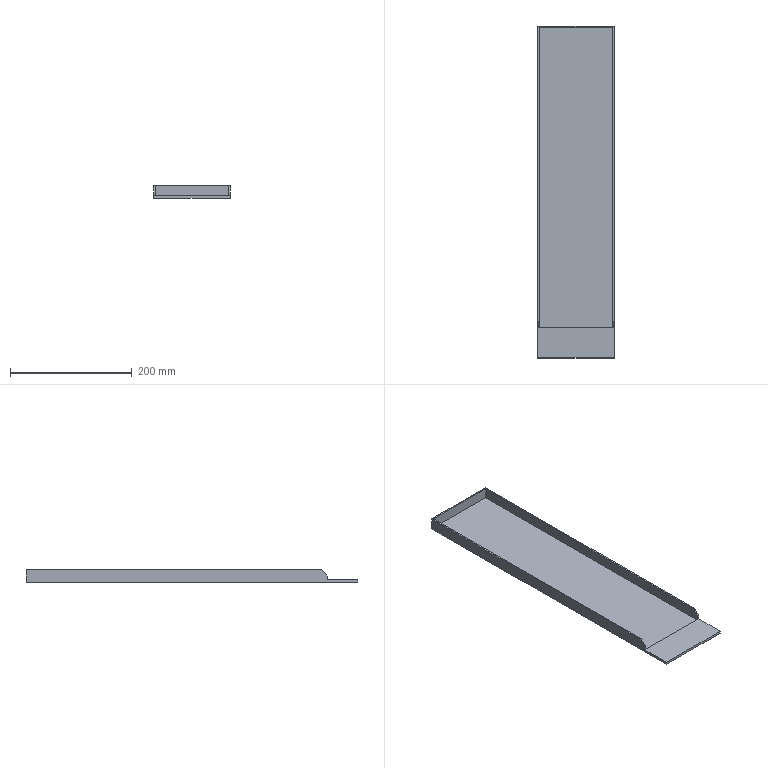Part | NX | features solid 2 | 1 solid | 16 faces | box 125 x 545 x 20 mm | volume 188546 mm3 | plane 16
STEP:
#1=CARTESIAN_POINT('',(-227.,-415.,-318.));
#2=VERTEX_POINT('',#1);
#3=CARTESIAN_POINT('',(-227.,78.,-318.));
#4=VERTEX_POINT('',#3);
#5=CARTESIAN_POINT('',(-227.,-415.,-318.));
#6=DIRECTION('',(0.,1.,0.));
#7=VECTOR('',#6,1000.);
#8=LINE('',#5,#7);
#9=EDGE_CURVE('',#2,#4,#8,.T.);
#10=ORIENTED_EDGE('',*,*,#9,.T.);
#11=CARTESIAN_POINT('',(-348.,78.,-318.));
#12=VERTEX_POINT('',#11);
#13=CARTESIAN_POINT('',(-350.,78.,-318.));
#14=DIRECTION('',(-1.,0.,0.));
#15=VECTOR('',#14,1000.);
#16=LINE('',#13,#15);
#17=EDGE_CURVE('',#12,#4,#16,.F.);
#18=ORIENTED_EDGE('',*,*,#17,.F.);
#19=CARTESIAN_POINT('',(-348.,-415.,-318.));
#20=VERTEX_POINT('',#19);
#21=CARTESIAN_POINT('',(-348.,78.,-318.));
#22=DIRECTION('',(0.,1.,0.));
#23=VECTOR('',#22,1000.);
#24=LINE('',#21,#23);
#25=EDGE_CURVE('',#12,#20,#24,.F.);
#26=ORIENTED_EDGE('',*,*,#25,.T.);
#27=CARTESIAN_POINT('',(-350.,-415.,-318.));
#28=DIRECTION('',(1.,0.,0.));
#29=VECTOR('',#28,1000.);
#30=LINE('',#27,#29);
#31=EDGE_CURVE('',#20,#2,#30,.T.);
#32=ORIENTED_EDGE('',*,*,#31,.T.);
#33=EDGE_LOOP('',(#10,#18,#26,#32));
#34=FACE_BOUND('',#33,.T.);
#35=CARTESIAN_POINT('',(-350.,-70.,-318.));
#36=DIRECTION('',(0.,0.,-1.));
#37=DIRECTION('',(-1.,0.,0.));
#38=AXIS2_PLACEMENT_3D('',#35,#36,#37);
#39=PLANE('',#38);
#40=ADVANCED_FACE('',(#34),#39,.F.);
#41=CARTESIAN_POINT('',(-225.,80.,-320.));
#42=VERTEX_POINT('',#41);
#43=CARTESIAN_POINT('',(-350.,80.,-320.));
#44=VERTEX_POINT('',#43);
#45=CARTESIAN_POINT('',(-350.,80.,-320.));
#46=DIRECTION('',(-1.,0.,0.));
#47=VECTOR('',#46,1000.);
#48=LINE('',#45,#47);
#49=EDGE_CURVE('',#42,#44,#48,.T.);
#50=ORIENTED_EDGE('',*,*,#49,.T.);
#51=CARTESIAN_POINT('',(-350.,80.,-300.));
#52=VERTEX_POINT('',#51);
#53=CARTESIAN_POINT('',(-350.,80.,-318.));
#54=DIRECTION('',(0.,0.,-1.));
#55=VECTOR('',#54,1000.);
#56=LINE('',#53,#55);
#57=EDGE_CURVE('',#52,#44,#56,.T.);
#58=ORIENTED_EDGE('',*,*,#57,.F.);
#59=CARTESIAN_POINT('',(-225.,80.,-300.));
#60=VERTEX_POINT('',#59);
#61=CARTESIAN_POINT('',(-380.,80.,-300.));
#62=DIRECTION('',(1.,0.,0.));
#63=VECTOR('',#62,1000.);
#64=LINE('',#61,#63);
#65=EDGE_CURVE('',#60,#52,#64,.F.);
#66=ORIENTED_EDGE('',*,*,#65,.F.);
#67=CARTESIAN_POINT('',(-225.,80.,-318.));
#68=DIRECTION('',(0.,0.,-1.));
#69=VECTOR('',#68,1000.);
#70=LINE('',#67,#69);
#71=EDGE_CURVE('',#60,#42,#70,.T.);
#72=ORIENTED_EDGE('',*,*,#71,.T.);
#73=EDGE_LOOP('',(#50,#58,#66,#72));
#74=FACE_BOUND('',#73,.T.);
#75=CARTESIAN_POINT('',(-350.,80.,-318.));
#76=DIRECTION('',(0.,-1.,0.));
#77=DIRECTION('',(0.,0.,-1.));
#78=AXIS2_PLACEMENT_3D('',#75,#76,#77);
#79=PLANE('',#78);
#80=ADVANCED_FACE('',(#74),#79,.F.);
#81=CARTESIAN_POINT('',(-225.,-405.,-300.));
#82=VERTEX_POINT('',#81);
#83=CARTESIAN_POINT('',(-225.,-15.,-300.));
#84=DIRECTION('',(0.,-1.,0.));
#85=VECTOR('',#84,1000.);
#86=LINE('',#83,#85);
#87=EDGE_CURVE('',#82,#60,#86,.F.);
#88=ORIENTED_EDGE('',*,*,#87,.F.);
#89=CARTESIAN_POINT('',(-225.,-415.,-310.));
#90=VERTEX_POINT('',#89);
#91=CARTESIAN_POINT('',(-225.,-415.,-310.));
#92=DIRECTION('',(0.,0.7071,0.7071));
#93=VECTOR('',#92,1000.);
#94=LINE('',#91,#93);
#95=EDGE_CURVE('',#82,#90,#94,.F.);
#96=ORIENTED_EDGE('',*,*,#95,.T.);
#97=CARTESIAN_POINT('',(-225.,-415.,-316.));
#98=VERTEX_POINT('',#97);
#99=CARTESIAN_POINT('',(-225.,-415.,-298.));
#100=DIRECTION('',(0.,0.,-1.));
#101=VECTOR('',#100,1000.);
#102=LINE('',#99,#101);
#103=EDGE_CURVE('',#90,#98,#102,.T.);
#104=ORIENTED_EDGE('',*,*,#103,.T.);
#105=CARTESIAN_POINT('',(-225.,-465.,-316.));
#106=VERTEX_POINT('',#105);
#107=CARTESIAN_POINT('',(-225.,-415.,-316.));
#108=DIRECTION('',(0.,1.,0.));
#109=VECTOR('',#108,1000.);
#110=LINE('',#107,#109);
#111=EDGE_CURVE('',#98,#106,#110,.F.);
#112=ORIENTED_EDGE('',*,*,#111,.T.);
#113=CARTESIAN_POINT('',(-225.,-465.,-320.));
#114=VERTEX_POINT('',#113);
#115=CARTESIAN_POINT('',(-225.,-465.,-318.));
#116=DIRECTION('',(0.,0.,1.));
#117=VECTOR('',#116,1000.);
#118=LINE('',#115,#117);
#119=EDGE_CURVE('',#106,#114,#118,.F.);
#120=ORIENTED_EDGE('',*,*,#119,.T.);
#121=CARTESIAN_POINT('',(-225.,-70.,-320.));
#122=DIRECTION('',(0.,-1.,0.));
#123=VECTOR('',#122,1000.);
#124=LINE('',#121,#123);
#125=EDGE_CURVE('',#114,#42,#124,.F.);
#126=ORIENTED_EDGE('',*,*,#125,.T.);
#127=ORIENTED_EDGE('',*,*,#71,.F.);
#128=EDGE_LOOP('',(#88,#96,#104,#112,#120,#126,#127));
#129=FACE_BOUND('',#128,.T.);
#130=CARTESIAN_POINT('',(-225.,-70.,-318.));
#131=DIRECTION('',(-1.,0.,0.));
#132=DIRECTION('',(0.,0.,1.));
#133=AXIS2_PLACEMENT_3D('',#130,#131,#132);
#134=PLANE('',#133);
#135=ADVANCED_FACE('',(#129),#134,.F.);
#136=CARTESIAN_POINT('',(-350.,-465.,-320.));
#137=VERTEX_POINT('',#136);
#138=CARTESIAN_POINT('',(-910.,-465.,-320.));
#139=DIRECTION('',(1.,0.,0.));
#140=VECTOR('',#139,1000.);
#141=LINE('',#138,#140);
#142=EDGE_CURVE('',#137,#114,#141,.T.);
#143=ORIENTED_EDGE('',*,*,#142,.T.);
#144=ORIENTED_EDGE('',*,*,#119,.F.);
#145=CARTESIAN_POINT('',(-350.,-465.,-316.));
#146=VERTEX_POINT('',#145);
#147=CARTESIAN_POINT('',(-350.,-465.,-316.));
#148=DIRECTION('',(-1.,0.,0.));
#149=VECTOR('',#148,1000.);
#150=LINE('',#147,#149);
#151=EDGE_CURVE('',#146,#106,#150,.F.);
#152=ORIENTED_EDGE('',*,*,#151,.F.);
#153=CARTESIAN_POINT('',(-350.,-465.,-85.));
#154=DIRECTION('',(0.,0.,1.));
#155=VECTOR('',#154,1000.);
#156=LINE('',#153,#155);
#157=EDGE_CURVE('',#146,#137,#156,.F.);
#158=ORIENTED_EDGE('',*,*,#157,.T.);
#159=EDGE_LOOP('',(#143,#144,#152,#158));
#160=FACE_BOUND('',#159,.T.);
#161=CARTESIAN_POINT('',(-910.,-465.,-85.));
#162=DIRECTION('',(0.,-1.,0.));
#163=DIRECTION('',(0.,0.,-1.));
#164=AXIS2_PLACEMENT_3D('',#161,#162,#163);
#165=PLANE('',#164);
#166=ADVANCED_FACE('',(#160),#165,.T.);
#167=CARTESIAN_POINT('',(-350.,-415.,-310.));
#168=VERTEX_POINT('',#167);
#169=CARTESIAN_POINT('',(-350.,-415.,-316.));
#170=VERTEX_POINT('',#169);
#171=CARTESIAN_POINT('',(-350.,-415.,-298.));
#172=DIRECTION('',(0.,0.,-1.));
#173=VECTOR('',#172,1000.);
#174=LINE('',#171,#173);
#175=EDGE_CURVE('',#168,#170,#174,.T.);
#176=ORIENTED_EDGE('',*,*,#175,.F.);
#177=CARTESIAN_POINT('',(-350.,-405.,-300.));
#178=VERTEX_POINT('',#177);
#179=CARTESIAN_POINT('',(-350.,-400.,-295.));
#180=DIRECTION('',(0.,0.7071,0.7071));
#181=VECTOR('',#180,1000.);
#182=LINE('',#179,#181);
#183=EDGE_CURVE('',#168,#178,#182,.T.);
#184=ORIENTED_EDGE('',*,*,#183,.T.);
#185=CARTESIAN_POINT('',(-350.,-70.,-300.));
#186=DIRECTION('',(0.,-1.,0.));
#187=VECTOR('',#186,1000.);
#188=LINE('',#185,#187);
#189=EDGE_CURVE('',#178,#52,#188,.F.);
#190=ORIENTED_EDGE('',*,*,#189,.T.);
#191=ORIENTED_EDGE('',*,*,#57,.T.);
#192=CARTESIAN_POINT('',(-350.,-70.,-320.));
#193=DIRECTION('',(0.,1.,0.));
#194=VECTOR('',#193,1000.);
#195=LINE('',#192,#194);
#196=EDGE_CURVE('',#44,#137,#195,.F.);
#197=ORIENTED_EDGE('',*,*,#196,.T.);
#198=ORIENTED_EDGE('',*,*,#157,.F.);
#199=CARTESIAN_POINT('',(-350.,-415.,-316.));
#200=DIRECTION('',(0.,1.,0.));
#201=VECTOR('',#200,1000.);
#202=LINE('',#199,#201);
#203=EDGE_CURVE('',#170,#146,#202,.F.);
#204=ORIENTED_EDGE('',*,*,#203,.F.);
#205=EDGE_LOOP('',(#176,#184,#190,#191,#197,#198,#204));
#206=FACE_BOUND('',#205,.T.);
#207=CARTESIAN_POINT('',(-350.,-70.,-318.));
#208=DIRECTION('',(1.,0.,0.));
#209=DIRECTION('',(0.,0.,-1.));
#210=AXIS2_PLACEMENT_3D('',#207,#208,#209);
#211=PLANE('',#210);
#212=ADVANCED_FACE('',(#206),#211,.F.);
#213=ORIENTED_EDGE('',*,*,#142,.F.);
#214=ORIENTED_EDGE('',*,*,#196,.F.);
#215=ORIENTED_EDGE('',*,*,#49,.F.);
#216=ORIENTED_EDGE('',*,*,#125,.F.);
#217=EDGE_LOOP('',(#213,#214,#215,#216));
#218=FACE_BOUND('',#217,.T.);
#219=CARTESIAN_POINT('',(-350.,-70.,-320.));
#220=DIRECTION('',(0.,0.,-1.));
#221=DIRECTION('',(-1.,0.,0.));
#222=AXIS2_PLACEMENT_3D('',#219,#220,#221);
#223=PLANE('',#222);
#224=ADVANCED_FACE('',(#218),#223,.T.);
#225=CARTESIAN_POINT('',(-227.,-415.,-316.));
#226=VERTEX_POINT('',#225);
#227=CARTESIAN_POINT('',(-227.,-415.,-298.));
#228=DIRECTION('',(0.,0.,1.));
#229=VECTOR('',#228,1000.);
#230=LINE('',#227,#229);
#231=EDGE_CURVE('',#226,#2,#230,.F.);
#232=ORIENTED_EDGE('',*,*,#231,.T.);
#233=ORIENTED_EDGE('',*,*,#31,.F.);
#234=CARTESIAN_POINT('',(-348.,-415.,-316.));
#235=VERTEX_POINT('',#234);
#236=CARTESIAN_POINT('',(-348.,-415.,-298.));
#237=DIRECTION('',(0.,0.,-1.));
#238=VECTOR('',#237,1000.);
#239=LINE('',#236,#238);
#240=EDGE_CURVE('',#235,#20,#239,.T.);
#241=ORIENTED_EDGE('',*,*,#240,.F.);
#242=CARTESIAN_POINT('',(-350.,-415.,-316.));
#243=DIRECTION('',(-1.,0.,0.));
#244=VECTOR('',#243,1000.);
#245=LINE('',#242,#244);
#246=EDGE_CURVE('',#235,#226,#245,.F.);
#247=ORIENTED_EDGE('',*,*,#246,.T.);
#248=EDGE_LOOP('',(#232,#233,#241,#247));
#249=FACE_BOUND('',#248,.T.);
#250=CARTESIAN_POINT('',(-350.,-415.,-318.));
#251=DIRECTION('',(0.,1.,0.));
#252=DIRECTION('',(1.,0.,0.));
#253=AXIS2_PLACEMENT_3D('',#250,#251,#252);
#254=PLANE('',#253);
#255=ADVANCED_FACE('',(#249),#254,.T.);
#256=ORIENTED_EDGE('',*,*,#151,.T.);
#257=ORIENTED_EDGE('',*,*,#111,.F.);
#258=CARTESIAN_POINT('',(-350.,-415.,-316.));
#259=DIRECTION('',(-1.,0.,0.));
#260=VECTOR('',#259,1000.);
#261=LINE('',#258,#260);
#262=EDGE_CURVE('',#226,#98,#261,.F.);
#263=ORIENTED_EDGE('',*,*,#262,.F.);
#264=ORIENTED_EDGE('',*,*,#246,.F.);
#265=CARTESIAN_POINT('',(-350.,-415.,-316.));
#266=DIRECTION('',(-1.,0.,0.));
#267=VECTOR('',#266,1000.);
#268=LINE('',#265,#267);
#269=EDGE_CURVE('',#170,#235,#268,.F.);
#270=ORIENTED_EDGE('',*,*,#269,.F.);
#271=ORIENTED_EDGE('',*,*,#203,.T.);
#272=EDGE_LOOP('',(#256,#257,#263,#264,#270,#271));
#273=FACE_BOUND('',#272,.T.);
#274=CARTESIAN_POINT('',(-350.,-415.,-316.));
#275=DIRECTION('',(0.,0.,-1.));
#276=DIRECTION('',(-1.,0.,0.));
#277=AXIS2_PLACEMENT_3D('',#274,#275,#276);
#278=PLANE('',#277);
#279=ADVANCED_FACE('',(#273),#278,.F.);
#280=CARTESIAN_POINT('',(-227.,78.,-300.));
#281=VERTEX_POINT('',#280);
#282=CARTESIAN_POINT('',(-227.,78.,-298.));
#283=DIRECTION('',(0.,0.,1.));
#284=VECTOR('',#283,1000.);
#285=LINE('',#282,#284);
#286=EDGE_CURVE('',#281,#4,#285,.F.);
#287=ORIENTED_EDGE('',*,*,#286,.F.);
#288=CARTESIAN_POINT('',(-348.,78.,-300.));
#289=VERTEX_POINT('',#288);
#290=CARTESIAN_POINT('',(-380.,78.,-300.));
#291=DIRECTION('',(1.,0.,0.));
#292=VECTOR('',#291,1000.);
#293=LINE('',#290,#292);
#294=EDGE_CURVE('',#281,#289,#293,.F.);
#295=ORIENTED_EDGE('',*,*,#294,.T.);
#296=CARTESIAN_POINT('',(-348.,78.,-298.));
#297=DIRECTION('',(0.,0.,-1.));
#298=VECTOR('',#297,1000.);
#299=LINE('',#296,#298);
#300=EDGE_CURVE('',#289,#12,#299,.T.);
#301=ORIENTED_EDGE('',*,*,#300,.T.);
#302=ORIENTED_EDGE('',*,*,#17,.T.);
#303=EDGE_LOOP('',(#287,#295,#301,#302));
#304=FACE_BOUND('',#303,.T.);
#305=CARTESIAN_POINT('',(-225.,78.,-318.));
#306=DIRECTION('',(0.,-1.,0.));
#307=DIRECTION('',(-1.,0.,0.));
#308=AXIS2_PLACEMENT_3D('',#305,#306,#307);
#309=PLANE('',#308);
#310=ADVANCED_FACE('',(#304),#309,.T.);
#311=CARTESIAN_POINT('',(-227.,-405.,-300.));
#312=VERTEX_POINT('',#311);
#313=CARTESIAN_POINT('',(-227.,-15.,-300.));
#314=DIRECTION('',(0.,-1.,0.));
#315=VECTOR('',#314,1000.);
#316=LINE('',#313,#315);
#317=EDGE_CURVE('',#312,#281,#316,.F.);
#318=ORIENTED_EDGE('',*,*,#317,.F.);
#319=CARTESIAN_POINT('',(-225.,-405.,-300.));
#320=DIRECTION('',(1.,0.,0.));
#321=VECTOR('',#320,1000.);
#322=LINE('',#319,#321);
#323=EDGE_CURVE('',#312,#82,#322,.T.);
#324=ORIENTED_EDGE('',*,*,#323,.T.);
#325=ORIENTED_EDGE('',*,*,#87,.T.);
#326=ORIENTED_EDGE('',*,*,#65,.T.);
#327=ORIENTED_EDGE('',*,*,#189,.F.);
#328=CARTESIAN_POINT('',(-348.,-405.,-300.));
#329=VERTEX_POINT('',#328);
#330=CARTESIAN_POINT('',(-225.,-405.,-300.));
#331=DIRECTION('',(-1.,0.,0.));
#332=VECTOR('',#331,1000.);
#333=LINE('',#330,#332);
#334=EDGE_CURVE('',#178,#329,#333,.F.);
#335=ORIENTED_EDGE('',*,*,#334,.T.);
#336=CARTESIAN_POINT('',(-348.,-15.,-300.));
#337=DIRECTION('',(0.,1.,0.));
#338=VECTOR('',#337,1000.);
#339=LINE('',#336,#338);
#340=EDGE_CURVE('',#289,#329,#339,.F.);
#341=ORIENTED_EDGE('',*,*,#340,.F.);
#342=ORIENTED_EDGE('',*,*,#294,.F.);
#343=EDGE_LOOP('',(#318,#324,#325,#326,#327,#335,#341,#342));
#344=FACE_BOUND('',#343,.T.);
#345=CARTESIAN_POINT('',(-380.,-15.,-300.));
#346=DIRECTION('',(0.,0.,1.));
#347=DIRECTION('',(1.,0.,0.));
#348=AXIS2_PLACEMENT_3D('',#345,#346,#347);
#349=PLANE('',#348);
#350=ADVANCED_FACE('',(#344),#349,.T.);
#351=CARTESIAN_POINT('',(-348.,-415.,-310.));
#352=VERTEX_POINT('',#351);
#353=CARTESIAN_POINT('',(-348.,-415.,-298.));
#354=DIRECTION('',(0.,0.,-1.));
#355=VECTOR('',#354,1000.);
#356=LINE('',#353,#355);
#357=EDGE_CURVE('',#352,#235,#356,.T.);
#358=ORIENTED_EDGE('',*,*,#357,.F.);
#359=CARTESIAN_POINT('',(-350.,-415.,-310.));
#360=DIRECTION('',(1.,0.,0.));
#361=VECTOR('',#360,1000.);
#362=LINE('',#359,#361);
#363=EDGE_CURVE('',#352,#168,#362,.F.);
#364=ORIENTED_EDGE('',*,*,#363,.T.);
#365=ORIENTED_EDGE('',*,*,#175,.T.);
#366=ORIENTED_EDGE('',*,*,#269,.T.);
#367=EDGE_LOOP('',(#358,#364,#365,#366));
#368=FACE_BOUND('',#367,.T.);
#369=CARTESIAN_POINT('',(-350.,-415.,-298.));
#370=DIRECTION('',(0.,-1.,0.));
#371=DIRECTION('',(0.,0.,-1.));
#372=AXIS2_PLACEMENT_3D('',#369,#370,#371);
#373=PLANE('',#372);
#374=ADVANCED_FACE('',(#368),#373,.T.);
#375=ORIENTED_EDGE('',*,*,#340,.T.);
#376=CARTESIAN_POINT('',(-348.,-162.5,-57.5));
#377=DIRECTION('',(0.,-0.7071,-0.7071));
#378=VECTOR('',#377,1000.);
#379=LINE('',#376,#378);
#380=EDGE_CURVE('',#329,#352,#379,.T.);
#381=ORIENTED_EDGE('',*,*,#380,.T.);
#382=ORIENTED_EDGE('',*,*,#357,.T.);
#383=ORIENTED_EDGE('',*,*,#240,.T.);
#384=ORIENTED_EDGE('',*,*,#25,.F.);
#385=ORIENTED_EDGE('',*,*,#300,.F.);
#386=EDGE_LOOP('',(#375,#381,#382,#383,#384,#385));
#387=FACE_BOUND('',#386,.T.);
#388=CARTESIAN_POINT('',(-348.,78.,-298.));
#389=DIRECTION('',(1.,0.,0.));
#390=DIRECTION('',(0.,0.,-1.));
#391=AXIS2_PLACEMENT_3D('',#388,#389,#390);
#392=PLANE('',#391);
#393=ADVANCED_FACE('',(#387),#392,.T.);
#394=ORIENTED_EDGE('',*,*,#103,.F.);
#395=CARTESIAN_POINT('',(-227.,-415.,-310.));
#396=VERTEX_POINT('',#395);
#397=CARTESIAN_POINT('',(-225.,-415.,-310.));
#398=DIRECTION('',(-1.,0.,0.));
#399=VECTOR('',#398,1000.);
#400=LINE('',#397,#399);
#401=EDGE_CURVE('',#90,#396,#400,.T.);
#402=ORIENTED_EDGE('',*,*,#401,.T.);
#403=CARTESIAN_POINT('',(-227.,-415.,-298.));
#404=DIRECTION('',(0.,0.,1.));
#405=VECTOR('',#404,1000.);
#406=LINE('',#403,#405);
#407=EDGE_CURVE('',#396,#226,#406,.F.);
#408=ORIENTED_EDGE('',*,*,#407,.T.);
#409=ORIENTED_EDGE('',*,*,#262,.T.);
#410=EDGE_LOOP('',(#394,#402,#408,#409));
#411=FACE_BOUND('',#410,.T.);
#412=CARTESIAN_POINT('',(-225.,-415.,-298.));
#413=DIRECTION('',(0.,1.,0.));
#414=DIRECTION('',(0.,0.,-1.));
#415=AXIS2_PLACEMENT_3D('',#412,#413,#414);
#416=PLANE('',#415);
#417=ADVANCED_FACE('',(#411),#416,.F.);
#418=ORIENTED_EDGE('',*,*,#407,.F.);
#419=CARTESIAN_POINT('',(-227.,-409.,-304.));
#420=DIRECTION('',(0.,-0.7071,-0.7071));
#421=VECTOR('',#420,1000.);
#422=LINE('',#419,#421);
#423=EDGE_CURVE('',#396,#312,#422,.F.);
#424=ORIENTED_EDGE('',*,*,#423,.T.);
#425=ORIENTED_EDGE('',*,*,#317,.T.);
#426=ORIENTED_EDGE('',*,*,#286,.T.);
#427=ORIENTED_EDGE('',*,*,#9,.F.);
#428=ORIENTED_EDGE('',*,*,#231,.F.);
#429=EDGE_LOOP('',(#418,#424,#425,#426,#427,#428));
#430=FACE_BOUND('',#429,.T.);
#431=CARTESIAN_POINT('',(-227.,-415.,-298.));
#432=DIRECTION('',(-1.,0.,0.));
#433=DIRECTION('',(0.,0.,1.));
#434=AXIS2_PLACEMENT_3D('',#431,#432,#433);
#435=PLANE('',#434);
#436=ADVANCED_FACE('',(#430),#435,.T.);
#437=ORIENTED_EDGE('',*,*,#183,.F.);
#438=ORIENTED_EDGE('',*,*,#363,.F.);
#439=ORIENTED_EDGE('',*,*,#380,.F.);
#440=ORIENTED_EDGE('',*,*,#334,.F.);
#441=EDGE_LOOP('',(#437,#438,#439,#440));
#442=FACE_BOUND('',#441,.T.);
#443=CARTESIAN_POINT('',(-225.,-400.,-295.));
#444=DIRECTION('',(0.,-0.7071,0.7071));
#445=DIRECTION('',(0.,-0.7071,-0.7071));
#446=AXIS2_PLACEMENT_3D('',#443,#444,#445);
#447=PLANE('',#446);
#448=ADVANCED_FACE('',(#442),#447,.T.);
#449=ORIENTED_EDGE('',*,*,#95,.F.);
#450=ORIENTED_EDGE('',*,*,#323,.F.);
#451=ORIENTED_EDGE('',*,*,#423,.F.);
#452=ORIENTED_EDGE('',*,*,#401,.F.);
#453=EDGE_LOOP('',(#449,#450,#451,#452));
#454=FACE_BOUND('',#453,.T.);
#455=CARTESIAN_POINT('',(-225.,-415.,-310.));
#456=DIRECTION('',(0.,0.7071,-0.7071));
#457=DIRECTION('',(0.,0.7071,0.7071));
#458=AXIS2_PLACEMENT_3D('',#455,#456,#457);
#459=PLANE('',#458);
#460=ADVANCED_FACE('',(#454),#459,.F.);
#461=CLOSED_SHELL('',(#40,#80,#135,#166,#212,#224,#255,#279,#310,#350,#374,#393,#417,#436,#448,#460));
#462=MANIFOLD_SOLID_BREP('',#461);
#463=(LENGTH_UNIT()NAMED_UNIT(*)SI_UNIT(.MILLI.,.METRE.));
#464=UNCERTAINTY_MEASURE_WITH_UNIT(LENGTH_MEASURE(0.00001),#463,'','');
#465=(NAMED_UNIT(*)PLANE_ANGLE_UNIT()SI_UNIT($,.RADIAN.));
#466=(NAMED_UNIT(*)SI_UNIT($,.STERADIAN.)SOLID_ANGLE_UNIT());
#467=(GEOMETRIC_REPRESENTATION_CONTEXT(3)GLOBAL_UNCERTAINTY_ASSIGNED_CONTEXT((#464))GLOBAL_UNIT_ASSIGNED_CONTEXT((#463,#465,#466))REPRESENTATION_CONTEXT('',''));
#468=ADVANCED_BREP_SHAPE_REPRESENTATION('',(#462),#467);